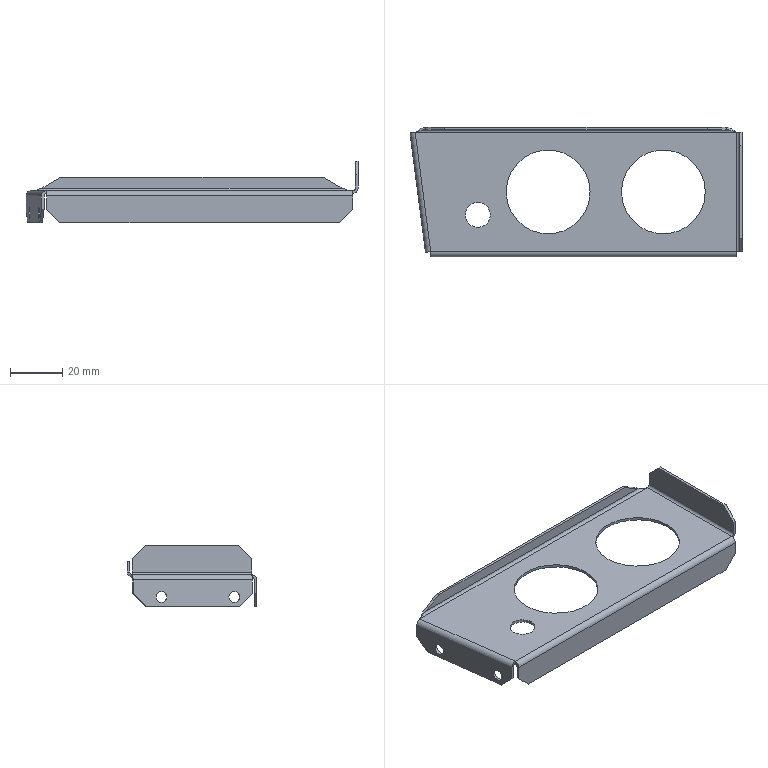Part | SolidWorks | features BaseBody 1 | 1 solid | 48 faces | box 126.707 x 49.5 x 23.288 mm | volume 6995 mm3 | plane 28 | cylinder 18 | spline 2 | commonest cylinder face diameters 2 x4 4 x4 4.17 x4 32 x4 9.5 x2